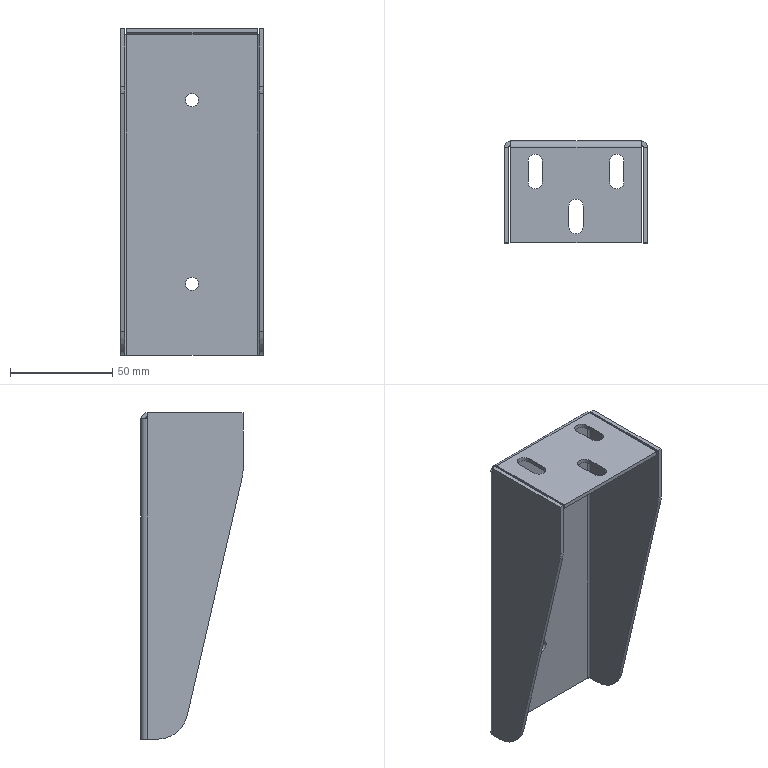Part | SolidWorks | features ICE 3, EdgeFlange 1, Fillet 1, FlatPattern 1, SMBaseFlange 1, SheetMetal 1 | 1 solid | 54 faces | box 70 x 50 x 160 mm | volume 49876 mm3 | plane 34 | cylinder 20 | commonest cylinder face diameters 7 x6 6.4 x4 30 x4 2 x3 6 x3
STEP:
#1=CARTESIAN_POINT('',(17.335,25.768,121.8));
#2=VERTEX_POINT('',#1);
#3=CARTESIAN_POINT('',(17.335,25.768,128.2));
#4=VERTEX_POINT('',#3);
#5=CARTESIAN_POINT('',(17.335,25.768,125.));
#6=DIRECTION('',(0.,1.,0.));
#7=DIRECTION('',(0.,0.,1.));
#8=AXIS2_PLACEMENT_3D('',#5,#6,#7);
#9=CIRCLE('',#8,3.2);
#10=EDGE_CURVE('',#2,#4,#9,.T.);
#11=ORIENTED_EDGE('',*,*,#10,.F.);
#12=CARTESIAN_POINT('',(17.335,27.768,121.8));
#13=VERTEX_POINT('',#12);
#14=CARTESIAN_POINT('',(17.335,-52.232,121.8));
#15=DIRECTION('',(0.,1.,0.));
#16=VECTOR('',#15,1000.);
#17=LINE('',#14,#16);
#18=EDGE_CURVE('',#2,#13,#17,.T.);
#19=ORIENTED_EDGE('',*,*,#18,.T.);
#20=CARTESIAN_POINT('',(17.335,27.768,128.2));
#21=VERTEX_POINT('',#20);
#22=CARTESIAN_POINT('',(17.335,27.768,125.));
#23=DIRECTION('',(0.,1.,0.));
#24=DIRECTION('',(0.,0.,1.));
#25=AXIS2_PLACEMENT_3D('',#22,#23,#24);
#26=CIRCLE('',#25,3.2);
#27=EDGE_CURVE('',#13,#21,#26,.T.);
#28=ORIENTED_EDGE('',*,*,#27,.T.);
#29=CARTESIAN_POINT('',(17.335,-52.232,128.2));
#30=DIRECTION('',(0.,1.,0.));
#31=VECTOR('',#30,1000.);
#32=LINE('',#29,#31);
#33=EDGE_CURVE('',#4,#21,#32,.T.);
#34=ORIENTED_EDGE('',*,*,#33,.F.);
#35=EDGE_LOOP('',(#11,#19,#28,#34));
#36=FACE_OUTER_BOUND('',#35,.T.);
#37=CARTESIAN_POINT('',(17.335,-52.232,125.));
#38=DIRECTION('',(0.,1.,0.));
#39=DIRECTION('',(0.,0.,1.));
#40=AXIS2_PLACEMENT_3D('',#37,#38,#39);
#41=CYLINDRICAL_SURFACE('',#40,3.2);
#42=ADVANCED_FACE('',(#36),#41,.F.);
#43=CARTESIAN_POINT('',(17.335,25.768,31.8));
#44=VERTEX_POINT('',#43);
#45=CARTESIAN_POINT('',(17.335,25.768,38.2));
#46=VERTEX_POINT('',#45);
#47=CARTESIAN_POINT('',(17.335,25.768,35.));
#48=DIRECTION('',(0.,1.,0.));
#49=DIRECTION('',(0.,0.,1.));
#50=AXIS2_PLACEMENT_3D('',#47,#48,#49);
#51=CIRCLE('',#50,3.2);
#52=EDGE_CURVE('',#44,#46,#51,.T.);
#53=ORIENTED_EDGE('',*,*,#52,.F.);
#54=CARTESIAN_POINT('',(17.335,27.768,31.8));
#55=VERTEX_POINT('',#54);
#56=CARTESIAN_POINT('',(17.335,-52.232,31.8));
#57=DIRECTION('',(0.,1.,0.));
#58=VECTOR('',#57,1000.);
#59=LINE('',#56,#58);
#60=EDGE_CURVE('',#44,#55,#59,.T.);
#61=ORIENTED_EDGE('',*,*,#60,.T.);
#62=CARTESIAN_POINT('',(17.335,27.768,38.2));
#63=VERTEX_POINT('',#62);
#64=CARTESIAN_POINT('',(17.335,27.768,35.));
#65=DIRECTION('',(0.,1.,0.));
#66=DIRECTION('',(0.,0.,1.));
#67=AXIS2_PLACEMENT_3D('',#64,#65,#66);
#68=CIRCLE('',#67,3.2);
#69=EDGE_CURVE('',#55,#63,#68,.T.);
#70=ORIENTED_EDGE('',*,*,#69,.T.);
#71=CARTESIAN_POINT('',(17.335,-52.232,38.2));
#72=DIRECTION('',(0.,1.,0.));
#73=VECTOR('',#72,1000.);
#74=LINE('',#71,#73);
#75=EDGE_CURVE('',#46,#63,#74,.T.);
#76=ORIENTED_EDGE('',*,*,#75,.F.);
#77=EDGE_LOOP('',(#53,#61,#70,#76));
#78=FACE_OUTER_BOUND('',#77,.T.);
#79=CARTESIAN_POINT('',(17.335,-52.232,35.));
#80=DIRECTION('',(0.,1.,0.));
#81=DIRECTION('',(0.,0.,1.));
#82=AXIS2_PLACEMENT_3D('',#79,#80,#81);
#83=CYLINDRICAL_SURFACE('',#82,3.2);
#84=ADVANCED_FACE('',(#78),#83,.F.);
#85=CARTESIAN_POINT('',(-15.665,19.701,0.));
#86=VERTEX_POINT('',#85);
#87=CARTESIAN_POINT('',(-15.665,24.768,0.));
#88=VERTEX_POINT('',#87);
#89=CARTESIAN_POINT('',(-15.665,-22.232,0.));
#90=DIRECTION('',(0.,1.,0.));
#91=VECTOR('',#90,1000.);
#92=LINE('',#89,#91);
#93=EDGE_CURVE('',#86,#88,#92,.T.);
#94=ORIENTED_EDGE('',*,*,#93,.F.);
#95=CARTESIAN_POINT('',(-17.665,19.701,0.));
#96=VERTEX_POINT('',#95);
#97=CARTESIAN_POINT('',(-14.665,19.701,0.));
#98=DIRECTION('',(-1.,0.,0.));
#99=VECTOR('',#98,1000.);
#100=LINE('',#97,#99);
#101=EDGE_CURVE('',#86,#96,#100,.T.);
#102=ORIENTED_EDGE('',*,*,#101,.T.);
#103=CARTESIAN_POINT('',(-17.665,24.768,0.));
#104=VERTEX_POINT('',#103);
#105=CARTESIAN_POINT('',(-17.665,-22.232,0.));
#106=DIRECTION('',(0.,1.,0.));
#107=VECTOR('',#106,1000.);
#108=LINE('',#105,#107);
#109=EDGE_CURVE('',#96,#104,#108,.T.);
#110=ORIENTED_EDGE('',*,*,#109,.T.);
#111=CARTESIAN_POINT('',(-17.665,24.768,0.));
#112=DIRECTION('',(1.,0.,0.));
#113=VECTOR('',#112,1000.);
#114=LINE('',#111,#113);
#115=EDGE_CURVE('',#104,#88,#114,.T.);
#116=ORIENTED_EDGE('',*,*,#115,.T.);
#117=EDGE_LOOP('',(#94,#102,#110,#116));
#118=FACE_OUTER_BOUND('',#117,.T.);
#119=CARTESIAN_POINT('',(-14.665,25.768,0.));
#120=DIRECTION('',(0.,0.,-1.));
#121=DIRECTION('',(-1.,0.,0.));
#122=AXIS2_PLACEMENT_3D('',#119,#120,#121);
#123=PLANE('',#122);
#124=ADVANCED_FACE('',(#118),#123,.T.);
#125=CARTESIAN_POINT('',(-17.665,-21.848,128.335));
#126=VERTEX_POINT('',#125);
#127=CARTESIAN_POINT('',(-17.665,5.085,11.627));
#128=VERTEX_POINT('',#127);
#129=CARTESIAN_POINT('',(-17.665,-28.805,158.483));
#130=DIRECTION('',(0.,0.2249,-0.9744));
#131=VECTOR('',#130,1000.);
#132=LINE('',#129,#131);
#133=EDGE_CURVE('',#126,#128,#132,.T.);
#134=ORIENTED_EDGE('',*,*,#133,.F.);
#135=CARTESIAN_POINT('',(-17.665,-22.232,131.708));
#136=VERTEX_POINT('',#135);
#137=CARTESIAN_POINT('',(-17.665,-7.232,131.708));
#138=DIRECTION('',(-1.,0.,0.));
#139=DIRECTION('',(0.,0.,1.));
#140=AXIS2_PLACEMENT_3D('',#137,#138,#139);
#141=CIRCLE('',#140,15.);
#142=EDGE_CURVE('',#126,#136,#141,.T.);
#143=ORIENTED_EDGE('',*,*,#142,.T.);
#144=CARTESIAN_POINT('',(-17.665,-22.232,160.));
#145=VERTEX_POINT('',#144);
#146=CARTESIAN_POINT('',(-17.665,-22.232,160.));
#147=DIRECTION('',(0.,0.,-1.));
#148=VECTOR('',#147,1000.);
#149=LINE('',#146,#148);
#150=EDGE_CURVE('',#145,#136,#149,.T.);
#151=ORIENTED_EDGE('',*,*,#150,.F.);
#152=CARTESIAN_POINT('',(-17.665,24.768,160.));
#153=VERTEX_POINT('',#152);
#154=CARTESIAN_POINT('',(-17.665,-22.232,160.));
#155=DIRECTION('',(0.,1.,0.));
#156=VECTOR('',#155,1000.);
#157=LINE('',#154,#156);
#158=EDGE_CURVE('',#145,#153,#157,.T.);
#159=ORIENTED_EDGE('',*,*,#158,.T.);
#160=CARTESIAN_POINT('',(-17.665,24.768,157.));
#161=VERTEX_POINT('',#160);
#162=CARTESIAN_POINT('',(-17.665,24.768,160.));
#163=DIRECTION('',(0.,0.,-1.));
#164=VECTOR('',#163,1000.);
#165=LINE('',#162,#164);
#166=EDGE_CURVE('',#153,#161,#165,.T.);
#167=ORIENTED_EDGE('',*,*,#166,.T.);
#168=CARTESIAN_POINT('',(-17.665,24.768,160.));
#169=DIRECTION('',(0.,0.,-1.));
#170=VECTOR('',#169,1000.);
#171=LINE('',#168,#170);
#172=EDGE_CURVE('',#161,#104,#171,.T.);
#173=ORIENTED_EDGE('',*,*,#172,.T.);
#174=ORIENTED_EDGE('',*,*,#109,.F.);
#175=CARTESIAN_POINT('',(-17.665,19.701,15.));
#176=DIRECTION('',(-1.,0.,0.));
#177=DIRECTION('',(0.,0.,1.));
#178=AXIS2_PLACEMENT_3D('',#175,#176,#177);
#179=CIRCLE('',#178,15.);
#180=EDGE_CURVE('',#96,#128,#179,.T.);
#181=ORIENTED_EDGE('',*,*,#180,.T.);
#182=EDGE_LOOP('',(#134,#143,#151,#159,#167,#173,#174,#181));
#183=FACE_OUTER_BOUND('',#182,.T.);
#184=CARTESIAN_POINT('',(-17.665,-22.232,160.));
#185=DIRECTION('',(-1.,0.,0.));
#186=DIRECTION('',(0.,0.,1.));
#187=AXIS2_PLACEMENT_3D('',#184,#185,#186);
#188=PLANE('',#187);
#189=ADVANCED_FACE('',(#183),#188,.T.);
#190=ORIENTED_EDGE('',*,*,#150,.T.);
#191=CARTESIAN_POINT('',(-15.665,-22.232,131.708));
#192=VERTEX_POINT('',#191);
#193=CARTESIAN_POINT('',(-15.665,-22.232,131.708));
#194=DIRECTION('',(1.,0.,0.));
#195=VECTOR('',#194,1000.);
#196=LINE('',#193,#195);
#197=EDGE_CURVE('',#136,#192,#196,.T.);
#198=ORIENTED_EDGE('',*,*,#197,.T.);
#199=CARTESIAN_POINT('',(-15.665,-22.232,160.));
#200=VERTEX_POINT('',#199);
#201=CARTESIAN_POINT('',(-15.665,-22.232,160.));
#202=DIRECTION('',(0.,0.,-1.));
#203=VECTOR('',#202,1000.);
#204=LINE('',#201,#203);
#205=EDGE_CURVE('',#200,#192,#204,.T.);
#206=ORIENTED_EDGE('',*,*,#205,.F.);
#207=CARTESIAN_POINT('',(-15.665,-22.232,160.));
#208=DIRECTION('',(-1.,0.,0.));
#209=VECTOR('',#208,1000.);
#210=LINE('',#207,#209);
#211=EDGE_CURVE('',#200,#145,#210,.T.);
#212=ORIENTED_EDGE('',*,*,#211,.T.);
#213=EDGE_LOOP('',(#190,#198,#206,#212));
#214=FACE_OUTER_BOUND('',#213,.T.);
#215=CARTESIAN_POINT('',(-15.665,-22.232,160.));
#216=DIRECTION('',(0.,-1.,0.));
#217=DIRECTION('',(0.,0.,-1.));
#218=AXIS2_PLACEMENT_3D('',#215,#216,#217);
#219=PLANE('',#218);
#220=ADVANCED_FACE('',(#214),#219,.T.);
#221=ORIENTED_EDGE('',*,*,#205,.T.);
#222=CARTESIAN_POINT('',(-15.665,-21.848,128.335));
#223=VERTEX_POINT('',#222);
#224=CARTESIAN_POINT('',(-15.665,-7.232,131.708));
#225=DIRECTION('',(1.,0.,0.));
#226=DIRECTION('',(0.,0.,1.));
#227=AXIS2_PLACEMENT_3D('',#224,#225,#226);
#228=CIRCLE('',#227,15.);
#229=EDGE_CURVE('',#192,#223,#228,.T.);
#230=ORIENTED_EDGE('',*,*,#229,.T.);
#231=CARTESIAN_POINT('',(-15.665,5.085,11.627));
#232=VERTEX_POINT('',#231);
#233=CARTESIAN_POINT('',(-15.665,-28.805,158.483));
#234=DIRECTION('',(0.,0.2249,-0.9744));
#235=VECTOR('',#234,1000.);
#236=LINE('',#233,#235);
#237=EDGE_CURVE('',#223,#232,#236,.T.);
#238=ORIENTED_EDGE('',*,*,#237,.T.);
#239=CARTESIAN_POINT('',(-15.665,19.701,15.));
#240=DIRECTION('',(1.,0.,0.));
#241=DIRECTION('',(0.,0.,1.));
#242=AXIS2_PLACEMENT_3D('',#239,#240,#241);
#243=CIRCLE('',#242,15.);
#244=EDGE_CURVE('',#232,#86,#243,.T.);
#245=ORIENTED_EDGE('',*,*,#244,.T.);
#246=ORIENTED_EDGE('',*,*,#93,.T.);
#247=CARTESIAN_POINT('',(-15.665,24.768,157.));
#248=VERTEX_POINT('',#247);
#249=CARTESIAN_POINT('',(-15.665,24.768,160.));
#250=DIRECTION('',(0.,0.,-1.));
#251=VECTOR('',#250,1000.);
#252=LINE('',#249,#251);
#253=EDGE_CURVE('',#248,#88,#252,.T.);
#254=ORIENTED_EDGE('',*,*,#253,.F.);
#255=CARTESIAN_POINT('',(-15.665,24.768,160.));
#256=VERTEX_POINT('',#255);
#257=CARTESIAN_POINT('',(-15.665,24.768,160.));
#258=DIRECTION('',(0.,0.,-1.));
#259=VECTOR('',#258,1000.);
#260=LINE('',#257,#259);
#261=EDGE_CURVE('',#256,#248,#260,.T.);
#262=ORIENTED_EDGE('',*,*,#261,.F.);
#263=CARTESIAN_POINT('',(-15.665,-22.232,160.));
#264=DIRECTION('',(0.,1.,0.));
#265=VECTOR('',#264,1000.);
#266=LINE('',#263,#265);
#267=EDGE_CURVE('',#200,#256,#266,.T.);
#268=ORIENTED_EDGE('',*,*,#267,.F.);
#269=EDGE_LOOP('',(#221,#230,#238,#245,#246,#254,#262,#268));
#270=FACE_OUTER_BOUND('',#269,.T.);
#271=CARTESIAN_POINT('',(-15.665,-22.232,160.));
#272=DIRECTION('',(-1.,0.,0.));
#273=DIRECTION('',(0.,0.,1.));
#274=AXIS2_PLACEMENT_3D('',#271,#272,#273);
#275=PLANE('',#274);
#276=ADVANCED_FACE('',(#270),#275,.F.);
#277=CARTESIAN_POINT('',(50.335,5.085,11.627));
#278=VERTEX_POINT('',#277);
#279=CARTESIAN_POINT('',(50.335,-21.848,128.335));
#280=VERTEX_POINT('',#279);
#281=CARTESIAN_POINT('',(50.335,-26.277,147.528));
#282=DIRECTION('',(0.,-0.2249,0.9744));
#283=VECTOR('',#282,1000.);
#284=LINE('',#281,#283);
#285=EDGE_CURVE('',#278,#280,#284,.T.);
#286=ORIENTED_EDGE('',*,*,#285,.T.);
#287=CARTESIAN_POINT('',(50.335,-22.232,131.708));
#288=VERTEX_POINT('',#287);
#289=CARTESIAN_POINT('',(50.335,-7.232,131.708));
#290=DIRECTION('',(-1.,0.,0.));
#291=DIRECTION('',(0.,1.,0.));
#292=AXIS2_PLACEMENT_3D('',#289,#290,#291);
#293=CIRCLE('',#292,15.);
#294=EDGE_CURVE('',#280,#288,#293,.T.);
#295=ORIENTED_EDGE('',*,*,#294,.T.);
#296=CARTESIAN_POINT('',(50.335,-22.232,160.));
#297=VERTEX_POINT('',#296);
#298=CARTESIAN_POINT('',(50.335,-22.232,160.));
#299=DIRECTION('',(0.,0.,-1.));
#300=VECTOR('',#299,1000.);
#301=LINE('',#298,#300);
#302=EDGE_CURVE('',#297,#288,#301,.T.);
#303=ORIENTED_EDGE('',*,*,#302,.F.);
#304=CARTESIAN_POINT('',(50.335,24.768,160.));
#305=VERTEX_POINT('',#304);
#306=CARTESIAN_POINT('',(50.335,27.768,160.));
#307=DIRECTION('',(0.,-1.,0.));
#308=VECTOR('',#307,1000.);
#309=LINE('',#306,#308);
#310=EDGE_CURVE('',#305,#297,#309,.T.);
#311=ORIENTED_EDGE('',*,*,#310,.F.);
#312=CARTESIAN_POINT('',(50.335,24.768,157.));
#313=VERTEX_POINT('',#312);
#314=CARTESIAN_POINT('',(50.335,24.768,160.));
#315=DIRECTION('',(0.,0.,-1.));
#316=VECTOR('',#315,1000.);
#317=LINE('',#314,#316);
#318=EDGE_CURVE('',#305,#313,#317,.T.);
#319=ORIENTED_EDGE('',*,*,#318,.T.);
#320=CARTESIAN_POINT('',(50.335,24.768,0.));
#321=VERTEX_POINT('',#320);
#322=CARTESIAN_POINT('',(50.335,24.768,160.));
#323=DIRECTION('',(0.,0.,-1.));
#324=VECTOR('',#323,1000.);
#325=LINE('',#322,#324);
#326=EDGE_CURVE('',#313,#321,#325,.T.);
#327=ORIENTED_EDGE('',*,*,#326,.T.);
#328=CARTESIAN_POINT('',(50.335,19.701,0.));
#329=VERTEX_POINT('',#328);
#330=CARTESIAN_POINT('',(50.335,27.768,0.));
#331=DIRECTION('',(0.,-1.,0.));
#332=VECTOR('',#331,1000.);
#333=LINE('',#330,#332);
#334=EDGE_CURVE('',#321,#329,#333,.T.);
#335=ORIENTED_EDGE('',*,*,#334,.T.);
#336=CARTESIAN_POINT('',(50.335,19.701,15.));
#337=DIRECTION('',(-1.,0.,0.));
#338=DIRECTION('',(0.,1.,0.));
#339=AXIS2_PLACEMENT_3D('',#336,#337,#338);
#340=CIRCLE('',#339,15.);
#341=EDGE_CURVE('',#329,#278,#340,.T.);
#342=ORIENTED_EDGE('',*,*,#341,.T.);
#343=EDGE_LOOP('',(#286,#295,#303,#311,#319,#327,#335,#342));
#344=FACE_OUTER_BOUND('',#343,.T.);
#345=CARTESIAN_POINT('',(50.335,27.768,160.));
#346=DIRECTION('',(1.,0.,0.));
#347=DIRECTION('',(0.,1.,0.));
#348=AXIS2_PLACEMENT_3D('',#345,#346,#347);
#349=PLANE('',#348);
#350=ADVANCED_FACE('',(#344),#349,.F.);
#351=ORIENTED_EDGE('',*,*,#302,.T.);
#352=CARTESIAN_POINT('',(52.335,-22.232,131.708));
#353=VERTEX_POINT('',#352);
#354=CARTESIAN_POINT('',(52.335,-22.232,131.708));
#355=DIRECTION('',(1.,0.,0.));
#356=VECTOR('',#355,1000.);
#357=LINE('',#354,#356);
#358=EDGE_CURVE('',#288,#353,#357,.T.);
#359=ORIENTED_EDGE('',*,*,#358,.T.);
#360=CARTESIAN_POINT('',(52.335,-22.232,160.));
#361=VERTEX_POINT('',#360);
#362=CARTESIAN_POINT('',(52.335,-22.232,160.));
#363=DIRECTION('',(0.,0.,-1.));
#364=VECTOR('',#363,1000.);
#365=LINE('',#362,#364);
#366=EDGE_CURVE('',#361,#353,#365,.T.);
#367=ORIENTED_EDGE('',*,*,#366,.F.);
#368=CARTESIAN_POINT('',(52.335,-22.232,160.));
#369=DIRECTION('',(-1.,0.,0.));
#370=VECTOR('',#369,1000.);
#371=LINE('',#368,#370);
#372=EDGE_CURVE('',#361,#297,#371,.T.);
#373=ORIENTED_EDGE('',*,*,#372,.T.);
#374=EDGE_LOOP('',(#351,#359,#367,#373));
#375=FACE_OUTER_BOUND('',#374,.T.);
#376=CARTESIAN_POINT('',(52.335,-22.232,160.));
#377=DIRECTION('',(0.,-1.,0.));
#378=DIRECTION('',(0.,0.,-1.));
#379=AXIS2_PLACEMENT_3D('',#376,#377,#378);
#380=PLANE('',#379);
#381=ADVANCED_FACE('',(#375),#380,.T.);
#382=ORIENTED_EDGE('',*,*,#366,.T.);
#383=CARTESIAN_POINT('',(52.335,-21.848,128.335));
#384=VERTEX_POINT('',#383);
#385=CARTESIAN_POINT('',(52.335,-7.232,131.708));
#386=DIRECTION('',(1.,0.,0.));
#387=DIRECTION('',(0.,1.,0.));
#388=AXIS2_PLACEMENT_3D('',#385,#386,#387);
#389=CIRCLE('',#388,15.);
#390=EDGE_CURVE('',#353,#384,#389,.T.);
#391=ORIENTED_EDGE('',*,*,#390,.T.);
#392=CARTESIAN_POINT('',(52.335,5.085,11.627));
#393=VERTEX_POINT('',#392);
#394=CARTESIAN_POINT('',(52.335,-26.277,147.528));
#395=DIRECTION('',(0.,-0.2249,0.9744));
#396=VECTOR('',#395,1000.);
#397=LINE('',#394,#396);
#398=EDGE_CURVE('',#393,#384,#397,.T.);
#399=ORIENTED_EDGE('',*,*,#398,.F.);
#400=CARTESIAN_POINT('',(52.335,19.701,0.));
#401=VERTEX_POINT('',#400);
#402=CARTESIAN_POINT('',(52.335,19.701,15.));
#403=DIRECTION('',(1.,0.,0.));
#404=DIRECTION('',(0.,1.,0.));
#405=AXIS2_PLACEMENT_3D('',#402,#403,#404);
#406=CIRCLE('',#405,15.);
#407=EDGE_CURVE('',#393,#401,#406,.T.);
#408=ORIENTED_EDGE('',*,*,#407,.T.);
#409=CARTESIAN_POINT('',(52.335,24.768,0.));
#410=VERTEX_POINT('',#409);
#411=CARTESIAN_POINT('',(52.335,27.768,0.));
#412=DIRECTION('',(0.,-1.,0.));
#413=VECTOR('',#412,1000.);
#414=LINE('',#411,#413);
#415=EDGE_CURVE('',#410,#401,#414,.T.);
#416=ORIENTED_EDGE('',*,*,#415,.F.);
#417=CARTESIAN_POINT('',(52.335,24.768,157.));
#418=VERTEX_POINT('',#417);
#419=CARTESIAN_POINT('',(52.335,24.768,160.));
#420=DIRECTION('',(0.,0.,-1.));
#421=VECTOR('',#420,1000.);
#422=LINE('',#419,#421);
#423=EDGE_CURVE('',#418,#410,#422,.T.);
#424=ORIENTED_EDGE('',*,*,#423,.F.);
#425=CARTESIAN_POINT('',(52.335,24.768,160.));
#426=VERTEX_POINT('',#425);
#427=CARTESIAN_POINT('',(52.335,24.768,160.));
#428=DIRECTION('',(0.,0.,-1.));
#429=VECTOR('',#428,1000.);
#430=LINE('',#427,#429);
#431=EDGE_CURVE('',#426,#418,#430,.T.);
#432=ORIENTED_EDGE('',*,*,#431,.F.);
#433=CARTESIAN_POINT('',(52.335,27.768,160.));
#434=DIRECTION('',(0.,-1.,0.));
#435=VECTOR('',#434,1000.);
#436=LINE('',#433,#435);
#437=EDGE_CURVE('',#426,#361,#436,.T.);
#438=ORIENTED_EDGE('',*,*,#437,.T.);
#439=EDGE_LOOP('',(#382,#391,#399,#408,#416,#424,#432,#438));
#440=FACE_OUTER_BOUND('',#439,.T.);
#441=CARTESIAN_POINT('',(52.335,27.768,160.));
#442=DIRECTION('',(1.,0.,0.));
#443=DIRECTION('',(0.,1.,0.));
#444=AXIS2_PLACEMENT_3D('',#441,#442,#443);
#445=PLANE('',#444);
#446=ADVANCED_FACE('',(#440),#445,.T.);
#447=ORIENTED_EDGE('',*,*,#415,.T.);
#448=CARTESIAN_POINT('',(50.335,19.701,0.));
#449=DIRECTION('',(-1.,0.,0.));
#450=VECTOR('',#449,1000.);
#451=LINE('',#448,#450);
#452=EDGE_CURVE('',#401,#329,#451,.T.);
#453=ORIENTED_EDGE('',*,*,#452,.T.);
#454=ORIENTED_EDGE('',*,*,#334,.F.);
#455=CARTESIAN_POINT('',(50.335,24.768,0.));
#456=DIRECTION('',(1.,0.,0.));
#457=VECTOR('',#456,1000.);
#458=LINE('',#455,#457);
#459=EDGE_CURVE('',#321,#410,#458,.T.);
#460=ORIENTED_EDGE('',*,*,#459,.T.);
#461=EDGE_LOOP('',(#447,#453,#454,#460));
#462=FACE_OUTER_BOUND('',#461,.T.);
#463=CARTESIAN_POINT('',(49.335,24.768,0.));
#464=DIRECTION('',(0.,0.,1.));
#465=DIRECTION('',(1.,0.,0.));
#466=AXIS2_PLACEMENT_3D('',#463,#464,#465);
#467=PLANE('',#466);
#468=ADVANCED_FACE('',(#462),#467,.F.);
#469=CARTESIAN_POINT('',(-17.665,24.768,157.));
#470=DIRECTION('',(1.,0.,0.));
#471=VECTOR('',#470,1000.);
#472=LINE('',#469,#471);
#473=EDGE_CURVE('',#161,#248,#472,.T.);
#474=ORIENTED_EDGE('',*,*,#473,.F.);
#475=ORIENTED_EDGE('',*,*,#166,.F.);
#476=CARTESIAN_POINT('',(-15.665,24.768,160.));
#477=DIRECTION('',(-1.,0.,0.));
#478=VECTOR('',#477,1000.);
#479=LINE('',#476,#478);
#480=EDGE_CURVE('',#256,#153,#479,.T.);
#481=ORIENTED_EDGE('',*,*,#480,.F.);
#482=ORIENTED_EDGE('',*,*,#261,.T.);
#483=EDGE_LOOP('',(#474,#475,#481,#482));
#484=FACE_OUTER_BOUND('',#483,.T.);
#485=CARTESIAN_POINT('',(0.,24.768,0.));
#486=DIRECTION('',(0.,1.,0.));
#487=DIRECTION('',(0.,0.,1.));
#488=AXIS2_PLACEMENT_3D('',#485,#486,#487);
#489=PLANE('',#488);
#490=ADVANCED_FACE('',(#484),#489,.T.);
#491=ORIENTED_EDGE('',*,*,#172,.F.);
#492=CARTESIAN_POINT('',(-14.665,27.768,157.));
#493=VERTEX_POINT('',#492);
#494=CARTESIAN_POINT('',(-14.665,24.768,157.));
#495=DIRECTION('',(0.,0.,-1.));
#496=DIRECTION('',(0.,-1.,0.));
#497=AXIS2_PLACEMENT_3D('',#494,#495,#496);
#498=CIRCLE('',#497,3.);
#499=EDGE_CURVE('',#161,#493,#498,.T.);
#500=ORIENTED_EDGE('',*,*,#499,.T.);
#501=CARTESIAN_POINT('',(-14.665,27.768,0.));
#502=VERTEX_POINT('',#501);
#503=CARTESIAN_POINT('',(-14.665,27.768,160.));
#504=DIRECTION('',(0.,0.,-1.));
#505=VECTOR('',#504,1000.);
#506=LINE('',#503,#505);
#507=EDGE_CURVE('',#493,#502,#506,.T.);
#508=ORIENTED_EDGE('',*,*,#507,.T.);
#509=CARTESIAN_POINT('',(-14.665,24.768,0.));
#510=DIRECTION('',(0.,0.,-1.));
#511=DIRECTION('',(1.,0.,0.));
#512=AXIS2_PLACEMENT_3D('',#509,#510,#511);
#513=CIRCLE('',#512,3.);
#514=EDGE_CURVE('',#104,#502,#513,.T.);
#515=ORIENTED_EDGE('',*,*,#514,.F.);
#516=EDGE_LOOP('',(#491,#500,#508,#515));
#517=FACE_OUTER_BOUND('',#516,.T.);
#518=CARTESIAN_POINT('',(-14.665,24.768,160.));
#519=DIRECTION('',(0.,0.,-1.));
#520=DIRECTION('',(-1.,0.,0.));
#521=AXIS2_PLACEMENT_3D('',#518,#519,#520);
#522=CYLINDRICAL_SURFACE('',#521,3.);
#523=ADVANCED_FACE('',(#517),#522,.T.);
#524=CARTESIAN_POINT('',(50.335,24.768,157.));
#525=DIRECTION('',(1.,0.,0.));
#526=VECTOR('',#525,1000.);
#527=LINE('',#524,#526);
#528=EDGE_CURVE('',#313,#418,#527,.T.);
#529=ORIENTED_EDGE('',*,*,#528,.F.);
#530=ORIENTED_EDGE('',*,*,#318,.F.);
#531=CARTESIAN_POINT('',(52.335,24.768,160.));
#532=DIRECTION('',(-1.,0.,0.));
#533=VECTOR('',#532,1000.);
#534=LINE('',#531,#533);
#535=EDGE_CURVE('',#426,#305,#534,.T.);
#536=ORIENTED_EDGE('',*,*,#535,.F.);
#537=ORIENTED_EDGE('',*,*,#431,.T.);
#538=EDGE_LOOP('',(#529,#530,#536,#537));
#539=FACE_OUTER_BOUND('',#538,.T.);
#540=CARTESIAN_POINT('',(0.,24.768,0.));
#541=DIRECTION('',(0.,1.,0.));
#542=DIRECTION('',(0.,0.,1.));
#543=AXIS2_PLACEMENT_3D('',#540,#541,#542);
#544=PLANE('',#543);
#545=ADVANCED_FACE('',(#539),#544,.T.);
#546=CARTESIAN_POINT('',(49.335,27.768,157.));
#547=VERTEX_POINT('',#546);
#548=CARTESIAN_POINT('',(49.335,27.768,0.));
#549=VERTEX_POINT('',#548);
#550=CARTESIAN_POINT('',(49.335,27.768,160.));
#551=DIRECTION('',(0.,0.,-1.));
#552=VECTOR('',#551,1000.);
#553=LINE('',#550,#552);
#554=EDGE_CURVE('',#547,#549,#553,.T.);
#555=ORIENTED_EDGE('',*,*,#554,.F.);
#556=CARTESIAN_POINT('',(49.335,24.768,157.));
#557=DIRECTION('',(0.,0.,-1.));
#558=DIRECTION('',(0.,-1.,0.));
#559=AXIS2_PLACEMENT_3D('',#556,#557,#558);
#560=CIRCLE('',#559,3.);
#561=EDGE_CURVE('',#547,#418,#560,.T.);
#562=ORIENTED_EDGE('',*,*,#561,.T.);
#563=ORIENTED_EDGE('',*,*,#423,.T.);
#564=CARTESIAN_POINT('',(49.335,24.768,0.));
#565=DIRECTION('',(0.,0.,-1.));
#566=DIRECTION('',(1.,0.,0.));
#567=AXIS2_PLACEMENT_3D('',#564,#565,#566);
#568=CIRCLE('',#567,3.);
#569=EDGE_CURVE('',#549,#410,#568,.T.);
#570=ORIENTED_EDGE('',*,*,#569,.F.);
#571=EDGE_LOOP('',(#555,#562,#563,#570));
#572=FACE_OUTER_BOUND('',#571,.T.);
#573=CARTESIAN_POINT('',(49.335,24.768,160.));
#574=DIRECTION('',(0.,0.,-1.));
#575=DIRECTION('',(-1.,0.,0.));
#576=AXIS2_PLACEMENT_3D('',#573,#574,#575);
#577=CYLINDRICAL_SURFACE('',#576,3.);
#578=ADVANCED_FACE('',(#572),#577,.T.);
#579=CARTESIAN_POINT('',(49.335,25.768,157.));
#580=VERTEX_POINT('',#579);
#581=CARTESIAN_POINT('',(49.335,24.768,157.));
#582=DIRECTION('',(0.,0.,-1.));
#583=DIRECTION('',(0.,-1.,0.));
#584=AXIS2_PLACEMENT_3D('',#581,#582,#583);
#585=CIRCLE('',#584,1.);
#586=EDGE_CURVE('',#580,#313,#585,.T.);
#587=ORIENTED_EDGE('',*,*,#586,.T.);
#588=ORIENTED_EDGE('',*,*,#528,.T.);
#589=ORIENTED_EDGE('',*,*,#561,.F.);
#590=CARTESIAN_POINT('',(49.335,25.768,157.));
#591=DIRECTION('',(0.,1.,0.));
#592=VECTOR('',#591,1000.);
#593=LINE('',#590,#592);
#594=EDGE_CURVE('',#580,#547,#593,.T.);
#595=ORIENTED_EDGE('',*,*,#594,.F.);
#596=EDGE_LOOP('',(#587,#588,#589,#595));
#597=FACE_OUTER_BOUND('',#596,.T.);
#598=CARTESIAN_POINT('',(49.335,24.768,157.));
#599=DIRECTION('',(0.,0.,1.));
#600=DIRECTION('',(0.,-1.,0.));
#601=AXIS2_PLACEMENT_3D('',#598,#599,#600);
#602=PLANE('',#601);
#603=ADVANCED_FACE('',(#597),#602,.T.);
#604=CARTESIAN_POINT('',(17.335,27.768,125.));
#605=DIRECTION('',(0.,1.,0.));
#606=DIRECTION('',(0.,0.,1.));
#607=AXIS2_PLACEMENT_3D('',#604,#605,#606);
#608=CIRCLE('',#607,3.2);
#609=EDGE_CURVE('',#21,#13,#608,.T.);
#610=ORIENTED_EDGE('',*,*,#609,.F.);
#611=ORIENTED_EDGE('',*,*,#27,.F.);
#612=EDGE_LOOP('',(#610,#611));
#613=FACE_BOUND('',#612,.T.);
#614=CARTESIAN_POINT('',(17.335,27.768,35.));
#615=DIRECTION('',(0.,1.,0.));
#616=DIRECTION('',(0.,0.,1.));
#617=AXIS2_PLACEMENT_3D('',#614,#615,#616);
#618=CIRCLE('',#617,3.2);
#619=EDGE_CURVE('',#63,#55,#618,.T.);
#620=ORIENTED_EDGE('',*,*,#619,.F.);
#621=ORIENTED_EDGE('',*,*,#69,.F.);
#622=EDGE_LOOP('',(#620,#621));
#623=FACE_BOUND('',#622,.T.);
#624=ORIENTED_EDGE('',*,*,#507,.F.);
#625=CARTESIAN_POINT('',(-14.665,27.768,157.));
#626=DIRECTION('',(1.,0.,0.));
#627=VECTOR('',#626,1000.);
#628=LINE('',#625,#627);
#629=EDGE_CURVE('',#493,#547,#628,.T.);
#630=ORIENTED_EDGE('',*,*,#629,.T.);
#631=ORIENTED_EDGE('',*,*,#554,.T.);
#632=CARTESIAN_POINT('',(-17.665,27.768,0.));
#633=DIRECTION('',(1.,0.,0.));
#634=VECTOR('',#633,1000.);
#635=LINE('',#632,#634);
#636=EDGE_CURVE('',#502,#549,#635,.T.);
#637=ORIENTED_EDGE('',*,*,#636,.F.);
#638=EDGE_LOOP('',(#624,#630,#631,#637));
#639=FACE_OUTER_BOUND('',#638,.T.);
#640=CARTESIAN_POINT('',(-17.665,27.768,160.));
#641=DIRECTION('',(0.,1.,0.));
#642=DIRECTION('',(0.,0.,1.));
#643=AXIS2_PLACEMENT_3D('',#640,#641,#642);
#644=PLANE('',#643);
#645=ADVANCED_FACE('',(#613,#623,#639),#644,.T.);
#646=CARTESIAN_POINT('',(17.335,25.768,125.));
#647=DIRECTION('',(0.,1.,0.));
#648=DIRECTION('',(0.,0.,1.));
#649=AXIS2_PLACEMENT_3D('',#646,#647,#648);
#650=CIRCLE('',#649,3.2);
#651=EDGE_CURVE('',#4,#2,#650,.T.);
#652=ORIENTED_EDGE('',*,*,#651,.T.);
#653=ORIENTED_EDGE('',*,*,#10,.T.);
#654=EDGE_LOOP('',(#652,#653));
#655=FACE_BOUND('',#654,.T.);
#656=CARTESIAN_POINT('',(17.335,25.768,35.));
#657=DIRECTION('',(0.,1.,0.));
#658=DIRECTION('',(0.,0.,1.));
#659=AXIS2_PLACEMENT_3D('',#656,#657,#658);
#660=CIRCLE('',#659,3.2);
#661=EDGE_CURVE('',#46,#44,#660,.T.);
#662=ORIENTED_EDGE('',*,*,#661,.T.);
#663=ORIENTED_EDGE('',*,*,#52,.T.);
#664=EDGE_LOOP('',(#662,#663));
#665=FACE_BOUND('',#664,.T.);
#666=CARTESIAN_POINT('',(-14.665,25.768,157.));
#667=VERTEX_POINT('',#666);
#668=CARTESIAN_POINT('',(-14.665,25.768,157.));
#669=DIRECTION('',(1.,0.,0.));
#670=VECTOR('',#669,1000.);
#671=LINE('',#668,#670);
#672=EDGE_CURVE('',#667,#580,#671,.T.);
#673=ORIENTED_EDGE('',*,*,#672,.F.);
#674=CARTESIAN_POINT('',(-14.665,25.768,0.));
#675=VERTEX_POINT('',#674);
#676=CARTESIAN_POINT('',(-14.665,25.768,160.));
#677=DIRECTION('',(0.,0.,-1.));
#678=VECTOR('',#677,1000.);
#679=LINE('',#676,#678);
#680=EDGE_CURVE('',#667,#675,#679,.T.);
#681=ORIENTED_EDGE('',*,*,#680,.T.);
#682=CARTESIAN_POINT('',(49.335,25.768,0.));
#683=VERTEX_POINT('',#682);
#684=CARTESIAN_POINT('',(-17.665,25.768,0.));
#685=DIRECTION('',(1.,0.,0.));
#686=VECTOR('',#685,1000.);
#687=LINE('',#684,#686);
#688=EDGE_CURVE('',#675,#683,#687,.T.);
#689=ORIENTED_EDGE('',*,*,#688,.T.);
#690=CARTESIAN_POINT('',(49.335,25.768,160.));
#691=DIRECTION('',(0.,0.,-1.));
#692=VECTOR('',#691,1000.);
#693=LINE('',#690,#692);
#694=EDGE_CURVE('',#580,#683,#693,.T.);
#695=ORIENTED_EDGE('',*,*,#694,.F.);
#696=EDGE_LOOP('',(#673,#681,#689,#695));
#697=FACE_OUTER_BOUND('',#696,.T.);
#698=CARTESIAN_POINT('',(-17.665,25.768,160.));
#699=DIRECTION('',(0.,1.,0.));
#700=DIRECTION('',(0.,0.,1.));
#701=AXIS2_PLACEMENT_3D('',#698,#699,#700);
#702=PLANE('',#701);
#703=ADVANCED_FACE('',(#655,#665,#697),#702,.F.);
#704=ORIENTED_EDGE('',*,*,#115,.F.);
#705=ORIENTED_EDGE('',*,*,#514,.T.);
#706=CARTESIAN_POINT('',(-14.665,25.768,0.));
#707=DIRECTION('',(0.,1.,0.));
#708=VECTOR('',#707,1000.);
#709=LINE('',#706,#708);
#710=EDGE_CURVE('',#675,#502,#709,.T.);
#711=ORIENTED_EDGE('',*,*,#710,.F.);
#712=CARTESIAN_POINT('',(-14.665,24.768,0.));
#713=DIRECTION('',(0.,0.,-1.));
#714=DIRECTION('',(1.,0.,0.));
#715=AXIS2_PLACEMENT_3D('',#712,#713,#714);
#716=CIRCLE('',#715,1.);
#717=EDGE_CURVE('',#88,#675,#716,.T.);
#718=ORIENTED_EDGE('',*,*,#717,.F.);
#719=EDGE_LOOP('',(#704,#705,#711,#718));
#720=FACE_OUTER_BOUND('',#719,.T.);
#721=CARTESIAN_POINT('',(-17.665,24.768,0.));
#722=DIRECTION('',(0.,0.,-1.));
#723=DIRECTION('',(-1.,0.,0.));
#724=AXIS2_PLACEMENT_3D('',#721,#722,#723);
#725=PLANE('',#724);
#726=ADVANCED_FACE('',(#720),#725,.T.);
#727=ORIENTED_EDGE('',*,*,#437,.F.);
#728=ORIENTED_EDGE('',*,*,#535,.T.);
#729=ORIENTED_EDGE('',*,*,#310,.T.);
#730=ORIENTED_EDGE('',*,*,#372,.F.);
#731=EDGE_LOOP('',(#727,#728,#729,#730));
#732=FACE_OUTER_BOUND('',#731,.T.);
#733=CARTESIAN_POINT('',(49.335,25.768,160.));
#734=DIRECTION('',(0.,0.,1.));
#735=DIRECTION('',(1.,0.,0.));
#736=AXIS2_PLACEMENT_3D('',#733,#734,#735);
#737=PLANE('',#736);
#738=ADVANCED_FACE('',(#732),#737,.T.);
#739=CARTESIAN_POINT('',(49.335,27.768,0.));
#740=DIRECTION('',(0.,-1.,0.));
#741=VECTOR('',#740,1000.);
#742=LINE('',#739,#741);
#743=EDGE_CURVE('',#549,#683,#742,.T.);
#744=ORIENTED_EDGE('',*,*,#743,.F.);
#745=ORIENTED_EDGE('',*,*,#569,.T.);
#746=ORIENTED_EDGE('',*,*,#459,.F.);
#747=CARTESIAN_POINT('',(49.335,24.768,0.));
#748=DIRECTION('',(0.,0.,-1.));
#749=DIRECTION('',(1.,0.,0.));
#750=AXIS2_PLACEMENT_3D('',#747,#748,#749);
#751=CIRCLE('',#750,1.);
#752=EDGE_CURVE('',#683,#321,#751,.T.);
#753=ORIENTED_EDGE('',*,*,#752,.F.);
#754=EDGE_LOOP('',(#744,#745,#746,#753));
#755=FACE_OUTER_BOUND('',#754,.T.);
#756=CARTESIAN_POINT('',(49.335,27.768,0.));
#757=DIRECTION('',(0.,0.,-1.));
#758=DIRECTION('',(-1.,0.,0.));
#759=AXIS2_PLACEMENT_3D('',#756,#757,#758);
#760=PLANE('',#759);
#761=ADVANCED_FACE('',(#755),#760,.T.);
#762=ORIENTED_EDGE('',*,*,#636,.T.);
#763=ORIENTED_EDGE('',*,*,#743,.T.);
#764=ORIENTED_EDGE('',*,*,#688,.F.);
#765=ORIENTED_EDGE('',*,*,#710,.T.);
#766=EDGE_LOOP('',(#762,#763,#764,#765));
#767=FACE_OUTER_BOUND('',#766,.T.);
#768=CARTESIAN_POINT('',(50.335,24.768,0.));
#769=DIRECTION('',(0.,0.,-1.));
#770=DIRECTION('',(-1.,0.,0.));
#771=AXIS2_PLACEMENT_3D('',#768,#769,#770);
#772=PLANE('',#771);
#773=ADVANCED_FACE('',(#767),#772,.T.);
#774=ORIENTED_EDGE('',*,*,#499,.F.);
#775=ORIENTED_EDGE('',*,*,#473,.T.);
#776=CARTESIAN_POINT('',(-14.665,24.768,157.));
#777=DIRECTION('',(0.,0.,-1.));
#778=DIRECTION('',(0.,-1.,0.));
#779=AXIS2_PLACEMENT_3D('',#776,#777,#778);
#780=CIRCLE('',#779,1.);
#781=EDGE_CURVE('',#248,#667,#780,.T.);
#782=ORIENTED_EDGE('',*,*,#781,.T.);
#783=CARTESIAN_POINT('',(-14.665,25.768,157.));
#784=DIRECTION('',(0.,1.,0.));
#785=VECTOR('',#784,1000.);
#786=LINE('',#783,#785);
#787=EDGE_CURVE('',#667,#493,#786,.T.);
#788=ORIENTED_EDGE('',*,*,#787,.T.);
#789=EDGE_LOOP('',(#774,#775,#782,#788));
#790=FACE_OUTER_BOUND('',#789,.T.);
#791=CARTESIAN_POINT('',(-14.665,24.768,157.));
#792=DIRECTION('',(0.,0.,1.));
#793=DIRECTION('',(0.,-1.,0.));
#794=AXIS2_PLACEMENT_3D('',#791,#792,#793);
#795=PLANE('',#794);
#796=ADVANCED_FACE('',(#790),#795,.T.);
#797=ORIENTED_EDGE('',*,*,#781,.F.);
#798=ORIENTED_EDGE('',*,*,#253,.T.);
#799=ORIENTED_EDGE('',*,*,#717,.T.);
#800=ORIENTED_EDGE('',*,*,#680,.F.);
#801=EDGE_LOOP('',(#797,#798,#799,#800));
#802=FACE_OUTER_BOUND('',#801,.T.);
#803=CARTESIAN_POINT('',(-14.665,24.768,160.));
#804=DIRECTION('',(0.,0.,-1.));
#805=DIRECTION('',(-1.,0.,0.));
#806=AXIS2_PLACEMENT_3D('',#803,#804,#805);
#807=CYLINDRICAL_SURFACE('',#806,1.);
#808=ADVANCED_FACE('',(#802),#807,.F.);
#809=ORIENTED_EDGE('',*,*,#586,.F.);
#810=ORIENTED_EDGE('',*,*,#694,.T.);
#811=ORIENTED_EDGE('',*,*,#752,.T.);
#812=ORIENTED_EDGE('',*,*,#326,.F.);
#813=EDGE_LOOP('',(#809,#810,#811,#812));
#814=FACE_OUTER_BOUND('',#813,.T.);
#815=CARTESIAN_POINT('',(49.335,24.768,160.));
#816=DIRECTION('',(0.,0.,-1.));
#817=DIRECTION('',(-1.,0.,0.));
#818=AXIS2_PLACEMENT_3D('',#815,#816,#817);
#819=CYLINDRICAL_SURFACE('',#818,1.);
#820=ADVANCED_FACE('',(#814),#819,.F.);
#821=ORIENTED_EDGE('',*,*,#267,.T.);
#822=ORIENTED_EDGE('',*,*,#480,.T.);
#823=ORIENTED_EDGE('',*,*,#158,.F.);
#824=ORIENTED_EDGE('',*,*,#211,.F.);
#825=EDGE_LOOP('',(#821,#822,#823,#824));
#826=FACE_OUTER_BOUND('',#825,.T.);
#827=CARTESIAN_POINT('',(49.335,24.768,160.));
#828=DIRECTION('',(0.,0.,1.));
#829=DIRECTION('',(1.,0.,0.));
#830=AXIS2_PLACEMENT_3D('',#827,#828,#829);
#831=PLANE('',#830);
#832=ADVANCED_FACE('',(#826),#831,.T.);
#833=CARTESIAN_POINT('',(49.335,24.768,158.));
#834=VERTEX_POINT('',#833);
#835=CARTESIAN_POINT('',(49.335,24.768,160.));
#836=VERTEX_POINT('',#835);
#837=CARTESIAN_POINT('',(49.335,24.768,160.));
#838=DIRECTION('',(0.,0.,1.));
#839=VECTOR('',#838,1000.);
#840=LINE('',#837,#839);
#841=EDGE_CURVE('',#834,#836,#840,.T.);
#842=ORIENTED_EDGE('',*,*,#841,.F.);
#843=CARTESIAN_POINT('',(49.335,24.768,157.));
#844=DIRECTION('',(1.,0.,0.));
#845=DIRECTION('',(0.,0.,1.));
#846=AXIS2_PLACEMENT_3D('',#843,#844,#845);
#847=CIRCLE('',#846,1.);
#848=EDGE_CURVE('',#580,#834,#847,.T.);
#849=ORIENTED_EDGE('',*,*,#848,.F.);
#850=ORIENTED_EDGE('',*,*,#594,.T.);
#851=CARTESIAN_POINT('',(49.335,24.768,157.));
#852=DIRECTION('',(1.,0.,0.));
#853=DIRECTION('',(0.,0.,1.));
#854=AXIS2_PLACEMENT_3D('',#851,#852,#853);
#855=CIRCLE('',#854,3.);
#856=EDGE_CURVE('',#547,#836,#855,.T.);
#857=ORIENTED_EDGE('',*,*,#856,.T.);
#858=EDGE_LOOP('',(#842,#849,#850,#857));
#859=FACE_OUTER_BOUND('',#858,.T.);
#860=CARTESIAN_POINT('',(49.335,24.768,157.));
#861=DIRECTION('',(1.,0.,0.));
#862=DIRECTION('',(0.,0.,-1.));
#863=AXIS2_PLACEMENT_3D('',#860,#861,#862);
#864=PLANE('',#863);
#865=ADVANCED_FACE('',(#859),#864,.T.);
#866=CARTESIAN_POINT('',(-14.665,24.768,158.));
#867=VERTEX_POINT('',#866);
#868=CARTESIAN_POINT('',(-14.665,24.768,157.));
#869=DIRECTION('',(-1.,0.,0.));
#870=DIRECTION('',(0.,0.,1.));
#871=AXIS2_PLACEMENT_3D('',#868,#869,#870);
#872=CIRCLE('',#871,1.);
#873=EDGE_CURVE('',#867,#667,#872,.T.);
#874=ORIENTED_EDGE('',*,*,#873,.F.);
#875=CARTESIAN_POINT('',(-14.665,24.768,160.));
#876=VERTEX_POINT('',#875);
#877=CARTESIAN_POINT('',(-14.665,24.768,158.));
#878=DIRECTION('',(0.,0.,1.));
#879=VECTOR('',#878,1000.);
#880=LINE('',#877,#879);
#881=EDGE_CURVE('',#867,#876,#880,.T.);
#882=ORIENTED_EDGE('',*,*,#881,.T.);
#883=CARTESIAN_POINT('',(-14.665,24.768,157.));
#884=DIRECTION('',(-1.,0.,0.));
#885=DIRECTION('',(0.,0.,1.));
#886=AXIS2_PLACEMENT_3D('',#883,#884,#885);
#887=CIRCLE('',#886,3.);
#888=EDGE_CURVE('',#876,#493,#887,.T.);
#889=ORIENTED_EDGE('',*,*,#888,.T.);
#890=ORIENTED_EDGE('',*,*,#787,.F.);
#891=EDGE_LOOP('',(#874,#882,#889,#890));
#892=FACE_OUTER_BOUND('',#891,.T.);
#893=CARTESIAN_POINT('',(-14.665,24.768,157.));
#894=DIRECTION('',(1.,0.,0.));
#895=DIRECTION('',(0.,0.,-1.));
#896=AXIS2_PLACEMENT_3D('',#893,#894,#895);
#897=PLANE('',#896);
#898=ADVANCED_FACE('',(#892),#897,.F.);
#899=ORIENTED_EDGE('',*,*,#629,.F.);
#900=ORIENTED_EDGE('',*,*,#888,.F.);
#901=CARTESIAN_POINT('',(0.,24.768,160.));
#902=DIRECTION('',(-1.,0.,0.));
#903=VECTOR('',#902,1000.);
#904=LINE('',#901,#903);
#905=EDGE_CURVE('',#836,#876,#904,.T.);
#906=ORIENTED_EDGE('',*,*,#905,.F.);
#907=ORIENTED_EDGE('',*,*,#856,.F.);
#908=EDGE_LOOP('',(#899,#900,#906,#907));
#909=FACE_OUTER_BOUND('',#908,.T.);
#910=CARTESIAN_POINT('',(-14.665,24.768,157.));
#911=DIRECTION('',(-1.,0.,0.));
#912=DIRECTION('',(0.,0.,1.));
#913=AXIS2_PLACEMENT_3D('',#910,#911,#912);
#914=CYLINDRICAL_SURFACE('',#913,3.);
#915=ADVANCED_FACE('',(#909),#914,.T.);
#916=ORIENTED_EDGE('',*,*,#672,.T.);
#917=ORIENTED_EDGE('',*,*,#848,.T.);
#918=CARTESIAN_POINT('',(49.335,24.768,158.));
#919=DIRECTION('',(-1.,0.,0.));
#920=VECTOR('',#919,1000.);
#921=LINE('',#918,#920);
#922=EDGE_CURVE('',#834,#867,#921,.T.);
#923=ORIENTED_EDGE('',*,*,#922,.T.);
#924=ORIENTED_EDGE('',*,*,#873,.T.);
#925=EDGE_LOOP('',(#916,#917,#923,#924));
#926=FACE_OUTER_BOUND('',#925,.T.);
#927=CARTESIAN_POINT('',(-14.665,24.768,157.));
#928=DIRECTION('',(-1.,0.,0.));
#929=DIRECTION('',(0.,0.,1.));
#930=AXIS2_PLACEMENT_3D('',#927,#928,#929);
#931=CYLINDRICAL_SURFACE('',#930,1.);
#932=ADVANCED_FACE('',(#926),#931,.F.);
#933=CARTESIAN_POINT('',(-14.665,-22.232,160.));
#934=VERTEX_POINT('',#933);
#935=CARTESIAN_POINT('',(-14.665,25.768,160.));
#936=DIRECTION('',(0.,1.,0.));
#937=VECTOR('',#936,1000.);
#938=LINE('',#935,#937);
#939=EDGE_CURVE('',#934,#876,#938,.T.);
#940=ORIENTED_EDGE('',*,*,#939,.T.);
#941=ORIENTED_EDGE('',*,*,#881,.F.);
#942=CARTESIAN_POINT('',(-14.665,-22.232,158.));
#943=VERTEX_POINT('',#942);
#944=CARTESIAN_POINT('',(-14.665,0.,158.));
#945=DIRECTION('',(0.,1.,0.));
#946=VECTOR('',#945,1000.);
#947=LINE('',#944,#946);
#948=EDGE_CURVE('',#943,#867,#947,.T.);
#949=ORIENTED_EDGE('',*,*,#948,.F.);
#950=CARTESIAN_POINT('',(-14.665,-22.232,160.));
#951=DIRECTION('',(0.,0.,-1.));
#952=VECTOR('',#951,1000.);
#953=LINE('',#950,#952);
#954=EDGE_CURVE('',#934,#943,#953,.T.);
#955=ORIENTED_EDGE('',*,*,#954,.F.);
#956=EDGE_LOOP('',(#940,#941,#949,#955));
#957=FACE_OUTER_BOUND('',#956,.T.);
#958=CARTESIAN_POINT('',(-14.665,25.768,160.));
#959=DIRECTION('',(-1.,0.,0.));
#960=DIRECTION('',(0.,-1.,0.));
#961=AXIS2_PLACEMENT_3D('',#958,#959,#960);
#962=PLANE('',#961);
#963=ADVANCED_FACE('',(#957),#962,.T.);
#964=CARTESIAN_POINT('',(49.335,-22.232,158.));
#965=VERTEX_POINT('',#964);
#966=CARTESIAN_POINT('',(49.335,0.,158.));
#967=DIRECTION('',(0.,-1.,0.));
#968=VECTOR('',#967,1000.);
#969=LINE('',#966,#968);
#970=EDGE_CURVE('',#834,#965,#969,.T.);
#971=ORIENTED_EDGE('',*,*,#970,.F.);
#972=ORIENTED_EDGE('',*,*,#841,.T.);
#973=CARTESIAN_POINT('',(49.335,-22.232,160.));
#974=VERTEX_POINT('',#973);
#975=CARTESIAN_POINT('',(49.335,-22.232,160.));
#976=DIRECTION('',(0.,-1.,0.));
#977=VECTOR('',#976,1000.);
#978=LINE('',#975,#977);
#979=EDGE_CURVE('',#836,#974,#978,.T.);
#980=ORIENTED_EDGE('',*,*,#979,.T.);
#981=CARTESIAN_POINT('',(49.335,-22.232,160.));
#982=DIRECTION('',(0.,0.,-1.));
#983=VECTOR('',#982,1000.);
#984=LINE('',#981,#983);
#985=EDGE_CURVE('',#974,#965,#984,.T.);
#986=ORIENTED_EDGE('',*,*,#985,.T.);
#987=EDGE_LOOP('',(#971,#972,#980,#986));
#988=FACE_OUTER_BOUND('',#987,.T.);
#989=CARTESIAN_POINT('',(49.335,-22.232,160.));
#990=DIRECTION('',(1.,0.,0.));
#991=DIRECTION('',(0.,0.,-1.));
#992=AXIS2_PLACEMENT_3D('',#989,#990,#991);
#993=PLANE('',#992);
#994=ADVANCED_FACE('',(#988),#993,.T.);
#995=CARTESIAN_POINT('',(40.835,17.768,160.));
#996=VERTEX_POINT('',#995);
#997=CARTESIAN_POINT('',(33.835,17.768,160.));
#998=VERTEX_POINT('',#997);
#999=CARTESIAN_POINT('',(37.335,17.768,160.));
#1000=DIRECTION('',(0.,0.,1.));
#1001=DIRECTION('',(1.,0.,0.));
#1002=AXIS2_PLACEMENT_3D('',#999,#1000,#1001);
#1003=CIRCLE('',#1002,3.5);
#1004=EDGE_CURVE('',#996,#998,#1003,.T.);
#1005=ORIENTED_EDGE('',*,*,#1004,.F.);
#1006=CARTESIAN_POINT('',(40.835,7.768,160.));
#1007=VERTEX_POINT('',#1006);
#1008=CARTESIAN_POINT('',(40.835,17.768,160.));
#1009=DIRECTION('',(0.,1.,0.));
#1010=VECTOR('',#1009,1000.);
#1011=LINE('',#1008,#1010);
#1012=EDGE_CURVE('',#1007,#996,#1011,.T.);
#1013=ORIENTED_EDGE('',*,*,#1012,.F.);
#1014=CARTESIAN_POINT('',(33.835,7.768,160.));
#1015=VERTEX_POINT('',#1014);
#1016=CARTESIAN_POINT('',(37.335,7.768,160.));
#1017=DIRECTION('',(0.,0.,1.));
#1018=DIRECTION('',(1.,0.,0.));
#1019=AXIS2_PLACEMENT_3D('',#1016,#1017,#1018);
#1020=CIRCLE('',#1019,3.5);
#1021=EDGE_CURVE('',#1015,#1007,#1020,.T.);
#1022=ORIENTED_EDGE('',*,*,#1021,.F.);
#1023=CARTESIAN_POINT('',(33.835,17.768,160.));
#1024=DIRECTION('',(0.,-1.,0.));
#1025=VECTOR('',#1024,1000.);
#1026=LINE('',#1023,#1025);
#1027=EDGE_CURVE('',#998,#1015,#1026,.T.);
#1028=ORIENTED_EDGE('',*,*,#1027,.F.);
#1029=EDGE_LOOP('',(#1005,#1013,#1022,#1028));
#1030=FACE_BOUND('',#1029,.T.);
#1031=CARTESIAN_POINT('',(20.835,-4.232,160.));
#1032=VERTEX_POINT('',#1031);
#1033=CARTESIAN_POINT('',(13.835,-4.232,160.));
#1034=VERTEX_POINT('',#1033);
#1035=CARTESIAN_POINT('',(17.335,-4.232,160.));
#1036=DIRECTION('',(0.,0.,1.));
#1037=DIRECTION('',(1.,0.,0.));
#1038=AXIS2_PLACEMENT_3D('',#1035,#1036,#1037);
#1039=CIRCLE('',#1038,3.5);
#1040=EDGE_CURVE('',#1032,#1034,#1039,.T.);
#1041=ORIENTED_EDGE('',*,*,#1040,.F.);
#1042=CARTESIAN_POINT('',(20.835,-14.232,160.));
#1043=VERTEX_POINT('',#1042);
#1044=CARTESIAN_POINT('',(20.835,-4.232,160.));
#1045=DIRECTION('',(0.,1.,0.));
#1046=VECTOR('',#1045,1000.);
#1047=LINE('',#1044,#1046);
#1048=EDGE_CURVE('',#1043,#1032,#1047,.T.);
#1049=ORIENTED_EDGE('',*,*,#1048,.F.);
#1050=CARTESIAN_POINT('',(13.835,-14.232,160.));
#1051=VERTEX_POINT('',#1050);
#1052=CARTESIAN_POINT('',(17.335,-14.232,160.));
#1053=DIRECTION('',(0.,0.,1.));
#1054=DIRECTION('',(1.,0.,0.));
#1055=AXIS2_PLACEMENT_3D('',#1052,#1053,#1054);
#1056=CIRCLE('',#1055,3.5);
#1057=EDGE_CURVE('',#1051,#1043,#1056,.T.);
#1058=ORIENTED_EDGE('',*,*,#1057,.F.);
#1059=CARTESIAN_POINT('',(13.835,-4.232,160.));
#1060=DIRECTION('',(0.,-1.,0.));
#1061=VECTOR('',#1060,1000.);
#1062=LINE('',#1059,#1061);
#1063=EDGE_CURVE('',#1034,#1051,#1062,.T.);
#1064=ORIENTED_EDGE('',*,*,#1063,.F.);
#1065=EDGE_LOOP('',(#1041,#1049,#1058,#1064));
#1066=FACE_BOUND('',#1065,.T.);
#1067=CARTESIAN_POINT('',(0.8349,17.768,160.));
#1068=VERTEX_POINT('',#1067);
#1069=CARTESIAN_POINT('',(-6.165,17.768,160.));
#1070=VERTEX_POINT('',#1069);
#1071=CARTESIAN_POINT('',(-2.665,17.768,160.));
#1072=DIRECTION('',(0.,0.,1.));
#1073=DIRECTION('',(1.,0.,0.));
#1074=AXIS2_PLACEMENT_3D('',#1071,#1072,#1073);
#1075=CIRCLE('',#1074,3.5);
#1076=EDGE_CURVE('',#1068,#1070,#1075,.T.);
#1077=ORIENTED_EDGE('',*,*,#1076,.F.);
#1078=CARTESIAN_POINT('',(0.8349,7.768,160.));
#1079=VERTEX_POINT('',#1078);
#1080=CARTESIAN_POINT('',(0.8349,17.768,160.));
#1081=DIRECTION('',(0.,1.,0.));
#1082=VECTOR('',#1081,1000.);
#1083=LINE('',#1080,#1082);
#1084=EDGE_CURVE('',#1079,#1068,#1083,.T.);
#1085=ORIENTED_EDGE('',*,*,#1084,.F.);
#1086=CARTESIAN_POINT('',(-6.165,7.768,160.));
#1087=VERTEX_POINT('',#1086);
#1088=CARTESIAN_POINT('',(-2.665,7.768,160.));
#1089=DIRECTION('',(0.,0.,1.));
#1090=DIRECTION('',(1.,0.,0.));
#1091=AXIS2_PLACEMENT_3D('',#1088,#1089,#1090);
#1092=CIRCLE('',#1091,3.5);
#1093=EDGE_CURVE('',#1087,#1079,#1092,.T.);
#1094=ORIENTED_EDGE('',*,*,#1093,.F.);
#1095=CARTESIAN_POINT('',(-6.165,17.768,160.));
#1096=DIRECTION('',(0.,-1.,0.));
#1097=VECTOR('',#1096,1000.);
#1098=LINE('',#1095,#1097);
#1099=EDGE_CURVE('',#1070,#1087,#1098,.T.);
#1100=ORIENTED_EDGE('',*,*,#1099,.F.);
#1101=EDGE_LOOP('',(#1077,#1085,#1094,#1100));
#1102=FACE_BOUND('',#1101,.T.);
#1103=ORIENTED_EDGE('',*,*,#979,.F.);
#1104=ORIENTED_EDGE('',*,*,#905,.T.);
#1105=ORIENTED_EDGE('',*,*,#939,.F.);
#1106=CARTESIAN_POINT('',(-14.665,-22.232,160.));
#1107=DIRECTION('',(-1.,0.,0.));
#1108=VECTOR('',#1107,1000.);
#1109=LINE('',#1106,#1108);
#1110=EDGE_CURVE('',#974,#934,#1109,.T.);
#1111=ORIENTED_EDGE('',*,*,#1110,.F.);
#1112=EDGE_LOOP('',(#1103,#1104,#1105,#1111));
#1113=FACE_OUTER_BOUND('',#1112,.T.);
#1114=CARTESIAN_POINT('',(0.,0.,160.));
#1115=DIRECTION('',(0.,0.,1.));
#1116=DIRECTION('',(0.,-1.,0.));
#1117=AXIS2_PLACEMENT_3D('',#1114,#1115,#1116);
#1118=PLANE('',#1117);
#1119=ADVANCED_FACE('',(#1030,#1066,#1102,#1113),#1118,.T.);
#1120=CARTESIAN_POINT('',(40.835,7.768,158.));
#1121=VERTEX_POINT('',#1120);
#1122=CARTESIAN_POINT('',(40.835,17.768,158.));
#1123=VERTEX_POINT('',#1122);
#1124=CARTESIAN_POINT('',(40.835,0.,158.));
#1125=DIRECTION('',(0.,1.,0.));
#1126=VECTOR('',#1125,1000.);
#1127=LINE('',#1124,#1126);
#1128=EDGE_CURVE('',#1121,#1123,#1127,.T.);
#1129=ORIENTED_EDGE('',*,*,#1128,.T.);
#1130=CARTESIAN_POINT('',(33.835,17.768,158.));
#1131=VERTEX_POINT('',#1130);
#1132=CARTESIAN_POINT('',(37.335,17.768,158.));
#1133=DIRECTION('',(0.,0.,1.));
#1134=DIRECTION('',(0.,-1.,0.));
#1135=AXIS2_PLACEMENT_3D('',#1132,#1133,#1134);
#1136=CIRCLE('',#1135,3.5);
#1137=EDGE_CURVE('',#1123,#1131,#1136,.T.);
#1138=ORIENTED_EDGE('',*,*,#1137,.T.);
#1139=CARTESIAN_POINT('',(33.835,7.768,158.));
#1140=VERTEX_POINT('',#1139);
#1141=CARTESIAN_POINT('',(33.835,0.,158.));
#1142=DIRECTION('',(0.,-1.,0.));
#1143=VECTOR('',#1142,1000.);
#1144=LINE('',#1141,#1143);
#1145=EDGE_CURVE('',#1131,#1140,#1144,.T.);
#1146=ORIENTED_EDGE('',*,*,#1145,.T.);
#1147=CARTESIAN_POINT('',(37.335,7.768,158.));
#1148=DIRECTION('',(0.,0.,1.));
#1149=DIRECTION('',(0.,-1.,0.));
#1150=AXIS2_PLACEMENT_3D('',#1147,#1148,#1149);
#1151=CIRCLE('',#1150,3.5);
#1152=EDGE_CURVE('',#1140,#1121,#1151,.T.);
#1153=ORIENTED_EDGE('',*,*,#1152,.T.);
#1154=EDGE_LOOP('',(#1129,#1138,#1146,#1153));
#1155=FACE_BOUND('',#1154,.T.);
#1156=CARTESIAN_POINT('',(20.835,-14.232,158.));
#1157=VERTEX_POINT('',#1156);
#1158=CARTESIAN_POINT('',(20.835,-4.232,158.));
#1159=VERTEX_POINT('',#1158);
#1160=CARTESIAN_POINT('',(20.835,0.,158.));
#1161=DIRECTION('',(0.,1.,0.));
#1162=VECTOR('',#1161,1000.);
#1163=LINE('',#1160,#1162);
#1164=EDGE_CURVE('',#1157,#1159,#1163,.T.);
#1165=ORIENTED_EDGE('',*,*,#1164,.T.);
#1166=CARTESIAN_POINT('',(13.835,-4.232,158.));
#1167=VERTEX_POINT('',#1166);
#1168=CARTESIAN_POINT('',(17.335,-4.232,158.));
#1169=DIRECTION('',(0.,0.,1.));
#1170=DIRECTION('',(0.,-1.,0.));
#1171=AXIS2_PLACEMENT_3D('',#1168,#1169,#1170);
#1172=CIRCLE('',#1171,3.5);
#1173=EDGE_CURVE('',#1159,#1167,#1172,.T.);
#1174=ORIENTED_EDGE('',*,*,#1173,.T.);
#1175=CARTESIAN_POINT('',(13.835,-14.232,158.));
#1176=VERTEX_POINT('',#1175);
#1177=CARTESIAN_POINT('',(13.835,0.,158.));
#1178=DIRECTION('',(0.,-1.,0.));
#1179=VECTOR('',#1178,1000.);
#1180=LINE('',#1177,#1179);
#1181=EDGE_CURVE('',#1167,#1176,#1180,.T.);
#1182=ORIENTED_EDGE('',*,*,#1181,.T.);
#1183=CARTESIAN_POINT('',(17.335,-14.232,158.));
#1184=DIRECTION('',(0.,0.,1.));
#1185=DIRECTION('',(0.,-1.,0.));
#1186=AXIS2_PLACEMENT_3D('',#1183,#1184,#1185);
#1187=CIRCLE('',#1186,3.5);
#1188=EDGE_CURVE('',#1176,#1157,#1187,.T.);
#1189=ORIENTED_EDGE('',*,*,#1188,.T.);
#1190=EDGE_LOOP('',(#1165,#1174,#1182,#1189));
#1191=FACE_BOUND('',#1190,.T.);
#1192=CARTESIAN_POINT('',(0.8349,7.768,158.));
#1193=VERTEX_POINT('',#1192);
#1194=CARTESIAN_POINT('',(0.8349,17.768,158.));
#1195=VERTEX_POINT('',#1194);
#1196=CARTESIAN_POINT('',(0.8349,0.,158.));
#1197=DIRECTION('',(0.,1.,0.));
#1198=VECTOR('',#1197,1000.);
#1199=LINE('',#1196,#1198);
#1200=EDGE_CURVE('',#1193,#1195,#1199,.T.);
#1201=ORIENTED_EDGE('',*,*,#1200,.T.);
#1202=CARTESIAN_POINT('',(-6.165,17.768,158.));
#1203=VERTEX_POINT('',#1202);
#1204=CARTESIAN_POINT('',(-2.665,17.768,158.));
#1205=DIRECTION('',(0.,0.,1.));
#1206=DIRECTION('',(0.,-1.,0.));
#1207=AXIS2_PLACEMENT_3D('',#1204,#1205,#1206);
#1208=CIRCLE('',#1207,3.5);
#1209=EDGE_CURVE('',#1195,#1203,#1208,.T.);
#1210=ORIENTED_EDGE('',*,*,#1209,.T.);
#1211=CARTESIAN_POINT('',(-6.165,7.768,158.));
#1212=VERTEX_POINT('',#1211);
#1213=CARTESIAN_POINT('',(-6.165,0.,158.));
#1214=DIRECTION('',(0.,-1.,0.));
#1215=VECTOR('',#1214,1000.);
#1216=LINE('',#1213,#1215);
#1217=EDGE_CURVE('',#1203,#1212,#1216,.T.);
#1218=ORIENTED_EDGE('',*,*,#1217,.T.);
#1219=CARTESIAN_POINT('',(-2.665,7.768,158.));
#1220=DIRECTION('',(0.,0.,1.));
#1221=DIRECTION('',(0.,-1.,0.));
#1222=AXIS2_PLACEMENT_3D('',#1219,#1220,#1221);
#1223=CIRCLE('',#1222,3.5);
#1224=EDGE_CURVE('',#1212,#1193,#1223,.T.);
#1225=ORIENTED_EDGE('',*,*,#1224,.T.);
#1226=EDGE_LOOP('',(#1201,#1210,#1218,#1225));
#1227=FACE_BOUND('',#1226,.T.);
#1228=ORIENTED_EDGE('',*,*,#922,.F.);
#1229=ORIENTED_EDGE('',*,*,#970,.T.);
#1230=CARTESIAN_POINT('',(0.,-22.232,158.));
#1231=DIRECTION('',(-1.,0.,0.));
#1232=VECTOR('',#1231,1000.);
#1233=LINE('',#1230,#1232);
#1234=EDGE_CURVE('',#965,#943,#1233,.T.);
#1235=ORIENTED_EDGE('',*,*,#1234,.T.);
#1236=ORIENTED_EDGE('',*,*,#948,.T.);
#1237=EDGE_LOOP('',(#1228,#1229,#1235,#1236));
#1238=FACE_OUTER_BOUND('',#1237,.T.);
#1239=CARTESIAN_POINT('',(0.,0.,158.));
#1240=DIRECTION('',(0.,0.,1.));
#1241=DIRECTION('',(0.,-1.,0.));
#1242=AXIS2_PLACEMENT_3D('',#1239,#1240,#1241);
#1243=PLANE('',#1242);
#1244=ADVANCED_FACE('',(#1155,#1191,#1227,#1238),#1243,.F.);
#1245=ORIENTED_EDGE('',*,*,#1234,.F.);
#1246=ORIENTED_EDGE('',*,*,#985,.F.);
#1247=ORIENTED_EDGE('',*,*,#1110,.T.);
#1248=ORIENTED_EDGE('',*,*,#954,.T.);
#1249=EDGE_LOOP('',(#1245,#1246,#1247,#1248));
#1250=FACE_OUTER_BOUND('',#1249,.T.);
#1251=CARTESIAN_POINT('',(-14.665,-22.232,160.));
#1252=DIRECTION('',(0.,-1.,0.));
#1253=DIRECTION('',(0.,0.,-1.));
#1254=AXIS2_PLACEMENT_3D('',#1251,#1252,#1253);
#1255=PLANE('',#1254);
#1256=ADVANCED_FACE('',(#1250),#1255,.T.);
#1257=ORIENTED_EDGE('',*,*,#398,.T.);
#1258=CARTESIAN_POINT('',(50.335,-21.848,128.335));
#1259=DIRECTION('',(-1.,0.,0.));
#1260=VECTOR('',#1259,1000.);
#1261=LINE('',#1258,#1260);
#1262=EDGE_CURVE('',#384,#280,#1261,.T.);
#1263=ORIENTED_EDGE('',*,*,#1262,.T.);
#1264=ORIENTED_EDGE('',*,*,#285,.F.);
#1265=CARTESIAN_POINT('',(52.335,5.085,11.627));
#1266=DIRECTION('',(1.,0.,0.));
#1267=VECTOR('',#1266,1000.);
#1268=LINE('',#1265,#1267);
#1269=EDGE_CURVE('',#278,#393,#1268,.T.);
#1270=ORIENTED_EDGE('',*,*,#1269,.T.);
#1271=EDGE_LOOP('',(#1257,#1263,#1264,#1270));
#1272=FACE_OUTER_BOUND('',#1271,.T.);
#1273=CARTESIAN_POINT('',(50.335,-26.277,147.528));
#1274=DIRECTION('',(0.,0.9744,0.2249));
#1275=DIRECTION('',(0.,-0.2249,0.9744));
#1276=AXIS2_PLACEMENT_3D('',#1273,#1274,#1275);
#1277=PLANE('',#1276);
#1278=ADVANCED_FACE('',(#1272),#1277,.F.);
#1279=ORIENTED_EDGE('',*,*,#237,.F.);
#1280=CARTESIAN_POINT('',(-17.665,-21.848,128.335));
#1281=DIRECTION('',(-1.,0.,0.));
#1282=VECTOR('',#1281,1000.);
#1283=LINE('',#1280,#1282);
#1284=EDGE_CURVE('',#223,#126,#1283,.T.);
#1285=ORIENTED_EDGE('',*,*,#1284,.T.);
#1286=ORIENTED_EDGE('',*,*,#133,.T.);
#1287=CARTESIAN_POINT('',(-17.665,5.085,11.627));
#1288=DIRECTION('',(1.,0.,0.));
#1289=VECTOR('',#1288,1000.);
#1290=LINE('',#1287,#1289);
#1291=EDGE_CURVE('',#128,#232,#1290,.T.);
#1292=ORIENTED_EDGE('',*,*,#1291,.T.);
#1293=EDGE_LOOP('',(#1279,#1285,#1286,#1292));
#1294=FACE_OUTER_BOUND('',#1293,.T.);
#1295=CARTESIAN_POINT('',(-17.665,-28.805,158.483));
#1296=DIRECTION('',(0.,0.9744,0.2249));
#1297=DIRECTION('',(0.,0.2249,-0.9744));
#1298=AXIS2_PLACEMENT_3D('',#1295,#1296,#1297);
#1299=PLANE('',#1298);
#1300=ADVANCED_FACE('',(#1294),#1299,.F.);
#1301=ORIENTED_EDGE('',*,*,#142,.F.);
#1302=ORIENTED_EDGE('',*,*,#1284,.F.);
#1303=ORIENTED_EDGE('',*,*,#229,.F.);
#1304=ORIENTED_EDGE('',*,*,#197,.F.);
#1305=EDGE_LOOP('',(#1301,#1302,#1303,#1304));
#1306=FACE_OUTER_BOUND('',#1305,.T.);
#1307=CARTESIAN_POINT('',(-15.665,-7.232,131.708));
#1308=DIRECTION('',(-1.,0.,0.));
#1309=DIRECTION('',(0.,0.,1.));
#1310=AXIS2_PLACEMENT_3D('',#1307,#1308,#1309);
#1311=CYLINDRICAL_SURFACE('',#1310,15.);
#1312=ADVANCED_FACE('',(#1306),#1311,.T.);
#1313=ORIENTED_EDGE('',*,*,#294,.F.);
#1314=ORIENTED_EDGE('',*,*,#1262,.F.);
#1315=ORIENTED_EDGE('',*,*,#390,.F.);
#1316=ORIENTED_EDGE('',*,*,#358,.F.);
#1317=EDGE_LOOP('',(#1313,#1314,#1315,#1316));
#1318=FACE_OUTER_BOUND('',#1317,.T.);
#1319=CARTESIAN_POINT('',(52.335,-7.232,131.708));
#1320=DIRECTION('',(-1.,0.,0.));
#1321=DIRECTION('',(0.,0.,1.));
#1322=AXIS2_PLACEMENT_3D('',#1319,#1320,#1321);
#1323=CYLINDRICAL_SURFACE('',#1322,15.);
#1324=ADVANCED_FACE('',(#1318),#1323,.T.);
#1325=ORIENTED_EDGE('',*,*,#180,.F.);
#1326=ORIENTED_EDGE('',*,*,#101,.F.);
#1327=ORIENTED_EDGE('',*,*,#244,.F.);
#1328=ORIENTED_EDGE('',*,*,#1291,.F.);
#1329=EDGE_LOOP('',(#1325,#1326,#1327,#1328));
#1330=FACE_OUTER_BOUND('',#1329,.T.);
#1331=CARTESIAN_POINT('',(-17.665,19.701,15.));
#1332=DIRECTION('',(-1.,0.,0.));
#1333=DIRECTION('',(0.,0.,1.));
#1334=AXIS2_PLACEMENT_3D('',#1331,#1332,#1333);
#1335=CYLINDRICAL_SURFACE('',#1334,15.);
#1336=ADVANCED_FACE('',(#1330),#1335,.T.);
#1337=ORIENTED_EDGE('',*,*,#341,.F.);
#1338=ORIENTED_EDGE('',*,*,#452,.F.);
#1339=ORIENTED_EDGE('',*,*,#407,.F.);
#1340=ORIENTED_EDGE('',*,*,#1269,.F.);
#1341=EDGE_LOOP('',(#1337,#1338,#1339,#1340));
#1342=FACE_OUTER_BOUND('',#1341,.T.);
#1343=CARTESIAN_POINT('',(50.335,19.701,15.));
#1344=DIRECTION('',(1.,0.,0.));
#1345=DIRECTION('',(0.,1.,0.));
#1346=AXIS2_PLACEMENT_3D('',#1343,#1344,#1345);
#1347=CYLINDRICAL_SURFACE('',#1346,15.);
#1348=ADVANCED_FACE('',(#1342),#1347,.T.);
#1349=ORIENTED_EDGE('',*,*,#60,.F.);
#1350=ORIENTED_EDGE('',*,*,#661,.F.);
#1351=ORIENTED_EDGE('',*,*,#75,.T.);
#1352=ORIENTED_EDGE('',*,*,#619,.T.);
#1353=EDGE_LOOP('',(#1349,#1350,#1351,#1352));
#1354=FACE_OUTER_BOUND('',#1353,.T.);
#1355=CARTESIAN_POINT('',(17.335,-52.232,35.));
#1356=DIRECTION('',(0.,1.,0.));
#1357=DIRECTION('',(0.,0.,1.));
#1358=AXIS2_PLACEMENT_3D('',#1355,#1356,#1357);
#1359=CYLINDRICAL_SURFACE('',#1358,3.2);
#1360=ADVANCED_FACE('',(#1354),#1359,.F.);
#1361=ORIENTED_EDGE('',*,*,#18,.F.);
#1362=ORIENTED_EDGE('',*,*,#651,.F.);
#1363=ORIENTED_EDGE('',*,*,#33,.T.);
#1364=ORIENTED_EDGE('',*,*,#609,.T.);
#1365=EDGE_LOOP('',(#1361,#1362,#1363,#1364));
#1366=FACE_OUTER_BOUND('',#1365,.T.);
#1367=CARTESIAN_POINT('',(17.335,-52.232,125.));
#1368=DIRECTION('',(0.,1.,0.));
#1369=DIRECTION('',(0.,0.,1.));
#1370=AXIS2_PLACEMENT_3D('',#1367,#1368,#1369);
#1371=CYLINDRICAL_SURFACE('',#1370,3.2);
#1372=ADVANCED_FACE('',(#1366),#1371,.F.);
#1373=CARTESIAN_POINT('',(0.8349,17.768,150.));
#1374=DIRECTION('',(0.,0.,1.));
#1375=VECTOR('',#1374,1000.);
#1376=LINE('',#1373,#1375);
#1377=EDGE_CURVE('',#1195,#1068,#1376,.T.);
#1378=ORIENTED_EDGE('',*,*,#1377,.T.);
#1379=ORIENTED_EDGE('',*,*,#1076,.T.);
#1380=CARTESIAN_POINT('',(-6.165,17.768,150.));
#1381=DIRECTION('',(0.,0.,1.));
#1382=VECTOR('',#1381,1000.);
#1383=LINE('',#1380,#1382);
#1384=EDGE_CURVE('',#1203,#1070,#1383,.T.);
#1385=ORIENTED_EDGE('',*,*,#1384,.F.);
#1386=ORIENTED_EDGE('',*,*,#1209,.F.);
#1387=EDGE_LOOP('',(#1378,#1379,#1385,#1386));
#1388=FACE_OUTER_BOUND('',#1387,.T.);
#1389=CARTESIAN_POINT('',(-2.665,17.768,150.));
#1390=DIRECTION('',(0.,0.,1.));
#1391=DIRECTION('',(1.,0.,0.));
#1392=AXIS2_PLACEMENT_3D('',#1389,#1390,#1391);
#1393=CYLINDRICAL_SURFACE('',#1392,3.5);
#1394=ADVANCED_FACE('',(#1388),#1393,.F.);
#1395=CARTESIAN_POINT('',(0.8349,7.768,150.));
#1396=DIRECTION('',(0.,0.,1.));
#1397=VECTOR('',#1396,1000.);
#1398=LINE('',#1395,#1397);
#1399=EDGE_CURVE('',#1193,#1079,#1398,.T.);
#1400=ORIENTED_EDGE('',*,*,#1399,.T.);
#1401=ORIENTED_EDGE('',*,*,#1084,.T.);
#1402=ORIENTED_EDGE('',*,*,#1377,.F.);
#1403=ORIENTED_EDGE('',*,*,#1200,.F.);
#1404=EDGE_LOOP('',(#1400,#1401,#1402,#1403));
#1405=FACE_OUTER_BOUND('',#1404,.T.);
#1406=CARTESIAN_POINT('',(0.8349,17.768,150.));
#1407=DIRECTION('',(1.,0.,0.));
#1408=DIRECTION('',(0.,0.,-1.));
#1409=AXIS2_PLACEMENT_3D('',#1406,#1407,#1408);
#1410=PLANE('',#1409);
#1411=ADVANCED_FACE('',(#1405),#1410,.F.);
#1412=CARTESIAN_POINT('',(-6.165,7.768,150.));
#1413=DIRECTION('',(0.,0.,1.));
#1414=VECTOR('',#1413,1000.);
#1415=LINE('',#1412,#1414);
#1416=EDGE_CURVE('',#1212,#1087,#1415,.T.);
#1417=ORIENTED_EDGE('',*,*,#1416,.T.);
#1418=ORIENTED_EDGE('',*,*,#1093,.T.);
#1419=ORIENTED_EDGE('',*,*,#1399,.F.);
#1420=ORIENTED_EDGE('',*,*,#1224,.F.);
#1421=EDGE_LOOP('',(#1417,#1418,#1419,#1420));
#1422=FACE_OUTER_BOUND('',#1421,.T.);
#1423=CARTESIAN_POINT('',(-2.665,7.768,150.));
#1424=DIRECTION('',(0.,0.,1.));
#1425=DIRECTION('',(1.,0.,0.));
#1426=AXIS2_PLACEMENT_3D('',#1423,#1424,#1425);
#1427=CYLINDRICAL_SURFACE('',#1426,3.5);
#1428=ADVANCED_FACE('',(#1422),#1427,.F.);
#1429=ORIENTED_EDGE('',*,*,#1384,.T.);
#1430=ORIENTED_EDGE('',*,*,#1099,.T.);
#1431=ORIENTED_EDGE('',*,*,#1416,.F.);
#1432=ORIENTED_EDGE('',*,*,#1217,.F.);
#1433=EDGE_LOOP('',(#1429,#1430,#1431,#1432));
#1434=FACE_OUTER_BOUND('',#1433,.T.);
#1435=CARTESIAN_POINT('',(-6.165,17.768,150.));
#1436=DIRECTION('',(-1.,0.,0.));
#1437=DIRECTION('',(0.,-1.,0.));
#1438=AXIS2_PLACEMENT_3D('',#1435,#1436,#1437);
#1439=PLANE('',#1438);
#1440=ADVANCED_FACE('',(#1434),#1439,.F.);
#1441=CARTESIAN_POINT('',(20.835,-4.232,150.));
#1442=DIRECTION('',(0.,0.,1.));
#1443=VECTOR('',#1442,1000.);
#1444=LINE('',#1441,#1443);
#1445=EDGE_CURVE('',#1159,#1032,#1444,.T.);
#1446=ORIENTED_EDGE('',*,*,#1445,.T.);
#1447=ORIENTED_EDGE('',*,*,#1040,.T.);
#1448=CARTESIAN_POINT('',(13.835,-4.232,150.));
#1449=DIRECTION('',(0.,0.,1.));
#1450=VECTOR('',#1449,1000.);
#1451=LINE('',#1448,#1450);
#1452=EDGE_CURVE('',#1167,#1034,#1451,.T.);
#1453=ORIENTED_EDGE('',*,*,#1452,.F.);
#1454=ORIENTED_EDGE('',*,*,#1173,.F.);
#1455=EDGE_LOOP('',(#1446,#1447,#1453,#1454));
#1456=FACE_OUTER_BOUND('',#1455,.T.);
#1457=CARTESIAN_POINT('',(17.335,-4.232,150.));
#1458=DIRECTION('',(0.,0.,1.));
#1459=DIRECTION('',(1.,0.,0.));
#1460=AXIS2_PLACEMENT_3D('',#1457,#1458,#1459);
#1461=CYLINDRICAL_SURFACE('',#1460,3.5);
#1462=ADVANCED_FACE('',(#1456),#1461,.F.);
#1463=CARTESIAN_POINT('',(20.835,-14.232,150.));
#1464=DIRECTION('',(0.,0.,1.));
#1465=VECTOR('',#1464,1000.);
#1466=LINE('',#1463,#1465);
#1467=EDGE_CURVE('',#1157,#1043,#1466,.T.);
#1468=ORIENTED_EDGE('',*,*,#1467,.T.);
#1469=ORIENTED_EDGE('',*,*,#1048,.T.);
#1470=ORIENTED_EDGE('',*,*,#1445,.F.);
#1471=ORIENTED_EDGE('',*,*,#1164,.F.);
#1472=EDGE_LOOP('',(#1468,#1469,#1470,#1471));
#1473=FACE_OUTER_BOUND('',#1472,.T.);
#1474=CARTESIAN_POINT('',(20.835,-4.232,150.));
#1475=DIRECTION('',(1.,0.,0.));
#1476=DIRECTION('',(0.,1.,0.));
#1477=AXIS2_PLACEMENT_3D('',#1474,#1475,#1476);
#1478=PLANE('',#1477);
#1479=ADVANCED_FACE('',(#1473),#1478,.F.);
#1480=CARTESIAN_POINT('',(13.835,-14.232,150.));
#1481=DIRECTION('',(0.,0.,1.));
#1482=VECTOR('',#1481,1000.);
#1483=LINE('',#1480,#1482);
#1484=EDGE_CURVE('',#1176,#1051,#1483,.T.);
#1485=ORIENTED_EDGE('',*,*,#1484,.T.);
#1486=ORIENTED_EDGE('',*,*,#1057,.T.);
#1487=ORIENTED_EDGE('',*,*,#1467,.F.);
#1488=ORIENTED_EDGE('',*,*,#1188,.F.);
#1489=EDGE_LOOP('',(#1485,#1486,#1487,#1488));
#1490=FACE_OUTER_BOUND('',#1489,.T.);
#1491=CARTESIAN_POINT('',(17.335,-14.232,150.));
#1492=DIRECTION('',(0.,0.,1.));
#1493=DIRECTION('',(1.,0.,0.));
#1494=AXIS2_PLACEMENT_3D('',#1491,#1492,#1493);
#1495=CYLINDRICAL_SURFACE('',#1494,3.5);
#1496=ADVANCED_FACE('',(#1490),#1495,.F.);
#1497=ORIENTED_EDGE('',*,*,#1452,.T.);
#1498=ORIENTED_EDGE('',*,*,#1063,.T.);
#1499=ORIENTED_EDGE('',*,*,#1484,.F.);
#1500=ORIENTED_EDGE('',*,*,#1181,.F.);
#1501=EDGE_LOOP('',(#1497,#1498,#1499,#1500));
#1502=FACE_OUTER_BOUND('',#1501,.T.);
#1503=CARTESIAN_POINT('',(13.835,-4.232,150.));
#1504=DIRECTION('',(-1.,0.,0.));
#1505=DIRECTION('',(0.,-1.,0.));
#1506=AXIS2_PLACEMENT_3D('',#1503,#1504,#1505);
#1507=PLANE('',#1506);
#1508=ADVANCED_FACE('',(#1502),#1507,.F.);
#1509=CARTESIAN_POINT('',(40.835,17.768,150.));
#1510=DIRECTION('',(0.,0.,1.));
#1511=VECTOR('',#1510,1000.);
#1512=LINE('',#1509,#1511);
#1513=EDGE_CURVE('',#1123,#996,#1512,.T.);
#1514=ORIENTED_EDGE('',*,*,#1513,.T.);
#1515=ORIENTED_EDGE('',*,*,#1004,.T.);
#1516=CARTESIAN_POINT('',(33.835,17.768,150.));
#1517=DIRECTION('',(0.,0.,1.));
#1518=VECTOR('',#1517,1000.);
#1519=LINE('',#1516,#1518);
#1520=EDGE_CURVE('',#1131,#998,#1519,.T.);
#1521=ORIENTED_EDGE('',*,*,#1520,.F.);
#1522=ORIENTED_EDGE('',*,*,#1137,.F.);
#1523=EDGE_LOOP('',(#1514,#1515,#1521,#1522));
#1524=FACE_OUTER_BOUND('',#1523,.T.);
#1525=CARTESIAN_POINT('',(37.335,17.768,150.));
#1526=DIRECTION('',(0.,0.,1.));
#1527=DIRECTION('',(1.,0.,0.));
#1528=AXIS2_PLACEMENT_3D('',#1525,#1526,#1527);
#1529=CYLINDRICAL_SURFACE('',#1528,3.5);
#1530=ADVANCED_FACE('',(#1524),#1529,.F.);
#1531=CARTESIAN_POINT('',(40.835,7.768,150.));
#1532=DIRECTION('',(0.,0.,1.));
#1533=VECTOR('',#1532,1000.);
#1534=LINE('',#1531,#1533);
#1535=EDGE_CURVE('',#1121,#1007,#1534,.T.);
#1536=ORIENTED_EDGE('',*,*,#1535,.T.);
#1537=ORIENTED_EDGE('',*,*,#1012,.T.);
#1538=ORIENTED_EDGE('',*,*,#1513,.F.);
#1539=ORIENTED_EDGE('',*,*,#1128,.F.);
#1540=EDGE_LOOP('',(#1536,#1537,#1538,#1539));
#1541=FACE_OUTER_BOUND('',#1540,.T.);
#1542=CARTESIAN_POINT('',(40.835,17.768,150.));
#1543=DIRECTION('',(1.,0.,0.));
#1544=DIRECTION('',(0.,0.,-1.));
#1545=AXIS2_PLACEMENT_3D('',#1542,#1543,#1544);
#1546=PLANE('',#1545);
#1547=ADVANCED_FACE('',(#1541),#1546,.F.);
#1548=CARTESIAN_POINT('',(33.835,7.768,150.));
#1549=DIRECTION('',(0.,0.,1.));
#1550=VECTOR('',#1549,1000.);
#1551=LINE('',#1548,#1550);
#1552=EDGE_CURVE('',#1140,#1015,#1551,.T.);
#1553=ORIENTED_EDGE('',*,*,#1552,.T.);
#1554=ORIENTED_EDGE('',*,*,#1021,.T.);
#1555=ORIENTED_EDGE('',*,*,#1535,.F.);
#1556=ORIENTED_EDGE('',*,*,#1152,.F.);
#1557=EDGE_LOOP('',(#1553,#1554,#1555,#1556));
#1558=FACE_OUTER_BOUND('',#1557,.T.);
#1559=CARTESIAN_POINT('',(37.335,7.768,150.));
#1560=DIRECTION('',(0.,0.,1.));
#1561=DIRECTION('',(1.,0.,0.));
#1562=AXIS2_PLACEMENT_3D('',#1559,#1560,#1561);
#1563=CYLINDRICAL_SURFACE('',#1562,3.5);
#1564=ADVANCED_FACE('',(#1558),#1563,.F.);
#1565=ORIENTED_EDGE('',*,*,#1520,.T.);
#1566=ORIENTED_EDGE('',*,*,#1027,.T.);
#1567=ORIENTED_EDGE('',*,*,#1552,.F.);
#1568=ORIENTED_EDGE('',*,*,#1145,.F.);
#1569=EDGE_LOOP('',(#1565,#1566,#1567,#1568));
#1570=FACE_OUTER_BOUND('',#1569,.T.);
#1571=CARTESIAN_POINT('',(33.835,17.768,150.));
#1572=DIRECTION('',(-1.,0.,0.));
#1573=DIRECTION('',(0.,0.,1.));
#1574=AXIS2_PLACEMENT_3D('',#1571,#1572,#1573);
#1575=PLANE('',#1574);
#1576=ADVANCED_FACE('',(#1570),#1575,.F.);
#1577=CLOSED_SHELL('',(#42,#84,#124,#189,#220,#276,#350,#381,#446,#468,#490,#523,#545,#578,#603,#645,#703,#726,#738,#761,#773,#796,#808,#820,#832,#865,#898,#915,#932,#963,#994,#1119,#1244,#1256,#1278,#1300,#1312,#1324,#1336,#1348,#1360,#1372,#1394,#1411,#1428,#1440,#1462,#1479,#1496,#1508,#1530,#1547,#1564,#1576));
#1578=MANIFOLD_SOLID_BREP('',#1577);
#1579=CARTESIAN_POINT('',(0.,0.,0.));
#1580=DIRECTION('',(0.,0.,1.));
#1581=DIRECTION('',(1.,0.,0.));
#1582=AXIS2_PLACEMENT_3D('',#1579,#1580,#1581);
#1583=(LENGTH_UNIT()NAMED_UNIT(*)SI_UNIT(.MILLI.,.METRE.));
#1584=UNCERTAINTY_MEASURE_WITH_UNIT(LENGTH_MEASURE(0.00001),#1583,'','');
#1585=(NAMED_UNIT(*)PLANE_ANGLE_UNIT()SI_UNIT($,.RADIAN.));
#1586=(NAMED_UNIT(*)SI_UNIT($,.STERADIAN.)SOLID_ANGLE_UNIT());
#1587=(GEOMETRIC_REPRESENTATION_CONTEXT(3)GLOBAL_UNCERTAINTY_ASSIGNED_CONTEXT((#1584))GLOBAL_UNIT_ASSIGNED_CONTEXT((#1583,#1585,#1586))REPRESENTATION_CONTEXT('',''));
#1588=ADVANCED_BREP_SHAPE_REPRESENTATION('',(#1578,#1582),#1587);